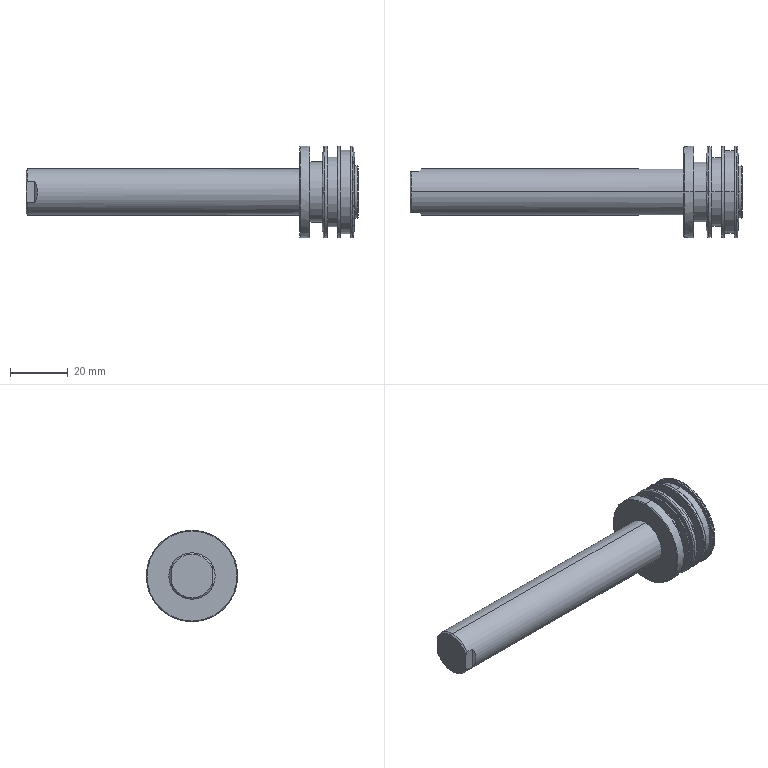Part | STEP file | TR_32x10-3 | 1 solid | 58 faces | box 114.8 x 31.6 x 31.6 mm | volume 30621 mm3 | cone 20 | cylinder 18 | plane 16 | spline 4 | commonest cylinder face diameters 31.6 x8 16 x2 18 x2 20.8 x2 24 x2 28.8 x2